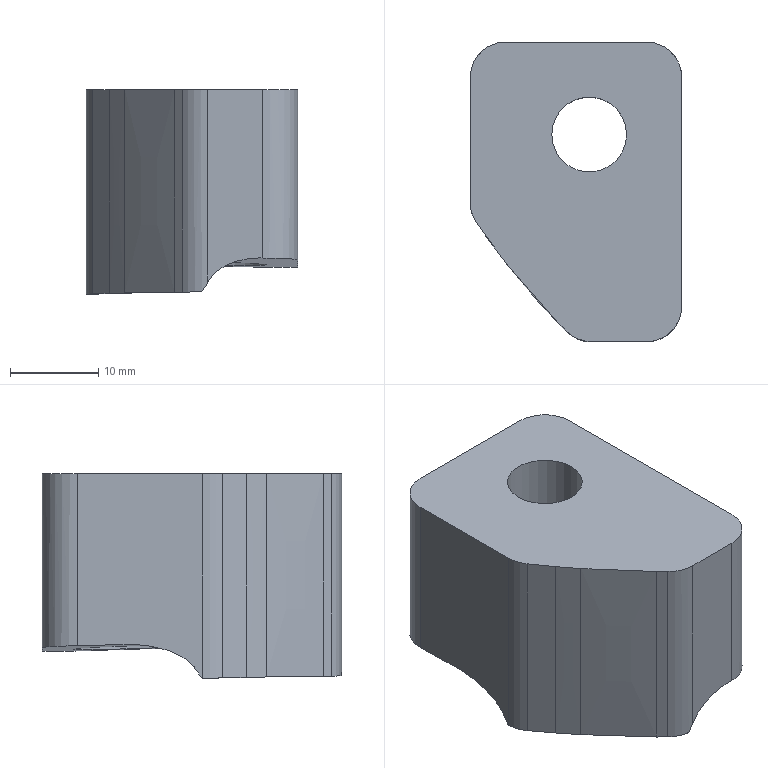Part | STEP file | gslz 2016.10.28-10_id1226_x_t | 1 solid | 21 faces | box 24 x 34 x 23.232 mm | volume 12031 mm3 | cylinder 7 | plane 6 | other 4 | spline 4 | commonest cylinder face diameters 8 x5 8.5 x1 14 x1